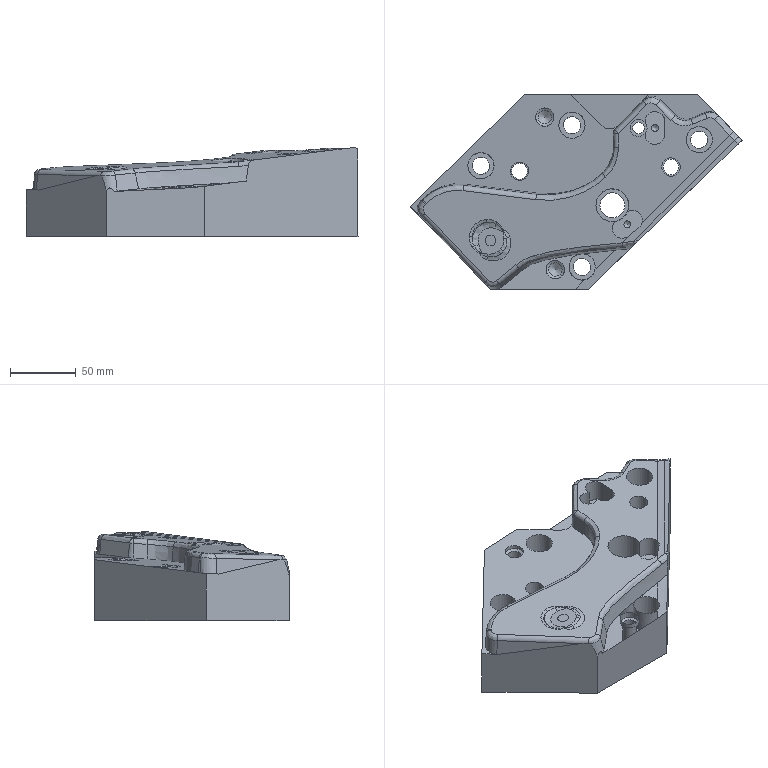Part | STEP file | 9805823380.1BPIECE_SOLIDE_FINALE_id1614_x_t | 1 solid | 137 faces | box 252.902 x 148 x 67.965 mm | volume 1153711 mm3 | spline 57 | cylinder 39 | plane 31 | cone 6 | other 3 | sphere 1 | commonest cylinder face diameters 7.5 x7 13 x5 14 x4 15 x4 20 x4 17.5 x3